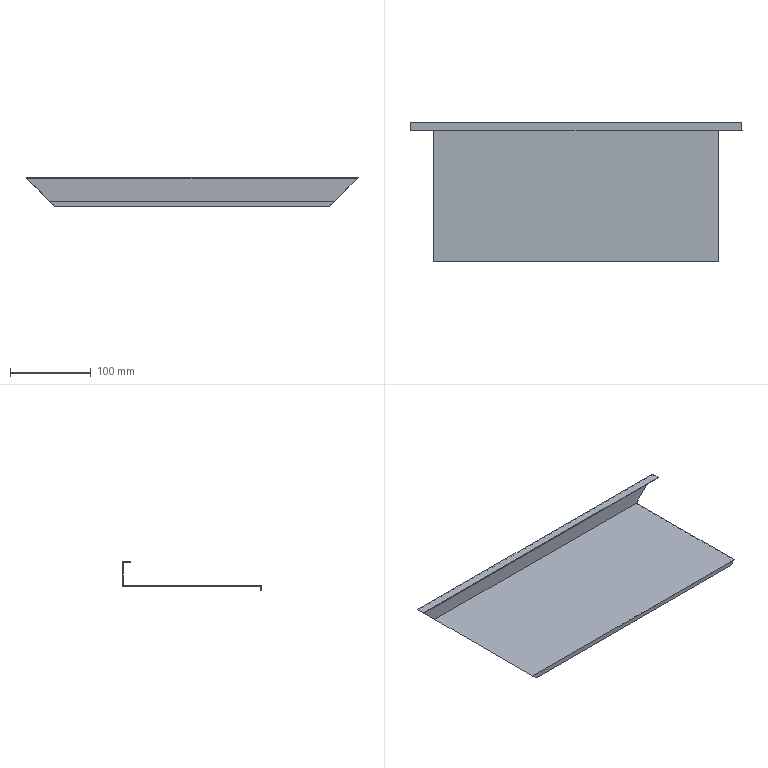Part | STEP file | 09-04 Inner side plate 1 | 1 solid | 12 faces | box 410 x 172 x 35 mm | volume 76827 mm3 | plane 12
STEP:
#1=CARTESIAN_POINT('',(0.,0.,0.));
#2=DIRECTION('',(0.,0.,1.));
#3=DIRECTION('',(1.,0.,0.));
#4=AXIS2_PLACEMENT_3D('',#1,#2,#3);
#5=CARTESIAN_POINT('',(381.,171.,1.));
#6=VERTEX_POINT('',#5);
#7=CARTESIAN_POINT('',(381.,0.,1.));
#8=VERTEX_POINT('',#7);
#9=CARTESIAN_POINT('',(381.,85.5,1.));
#10=DIRECTION('',(0.,-1.,0.));
#11=VECTOR('',#10,1.);
#12=LINE('',#9,#11);
#13=CARTESIAN_POINT('',(29.,0.,1.));
#14=DIRECTION('',(0.,0.,-1.));
#15=DIRECTION('',(0.,1.,0.));
#16=AXIS2_PLACEMENT_3D('',#13,#14,#15);
#17=PLANE('',#16);
#18=CARTESIAN_POINT('',(85.5,352.));
#19=DIRECTION('',(-1.,0.));
#20=VECTOR('',#19,1.);
#21=LINE('',#18,#20);
#22=(GEOMETRIC_REPRESENTATION_CONTEXT(2)PARAMETRIC_REPRESENTATION_CONTEXT()REPRESENTATION_CONTEXT('',''));
#23=DEFINITIONAL_REPRESENTATION('',(#21),#22);
#24=PCURVE('',#17,#23);
#25=CARTESIAN_POINT('',(375.,0.,-5.));
#26=DIRECTION('',(-0.7071,0.,0.7071));
#27=DIRECTION('',(0.7071,0.,0.7071));
#28=AXIS2_PLACEMENT_3D('',#25,#26,#27);
#29=PLANE('',#28);
#30=CARTESIAN_POINT('',(8.485,85.5));
#31=DIRECTION('',(0.,-1.));
#32=VECTOR('',#31,1.);
#33=LINE('',#30,#32);
#34=(GEOMETRIC_REPRESENTATION_CONTEXT(2)PARAMETRIC_REPRESENTATION_CONTEXT()REPRESENTATION_CONTEXT('',''));
#35=DEFINITIONAL_REPRESENTATION('',(#33),#34);
#36=PCURVE('',#29,#35);
#37=SURFACE_CURVE('',#12,(#24,#36),.PCURVE_S1.);
#38=EDGE_CURVE('',#6,#8,#37,.T.);
#39=ORIENTED_EDGE('',*,*,#38,.F.);
#40=CARTESIAN_POINT('',(29.,171.,1.));
#41=VERTEX_POINT('',#40);
#42=CARTESIAN_POINT('',(205.,171.,1.));
#43=DIRECTION('',(1.,0.,0.));
#44=VECTOR('',#43,1.);
#45=LINE('',#42,#44);
#46=CARTESIAN_POINT('',(171.,176.));
#47=DIRECTION('',(0.,1.));
#48=VECTOR('',#47,1.);
#49=LINE('',#46,#48);
#50=(GEOMETRIC_REPRESENTATION_CONTEXT(2)PARAMETRIC_REPRESENTATION_CONTEXT()REPRESENTATION_CONTEXT('',''));
#51=DEFINITIONAL_REPRESENTATION('',(#49),#50);
#52=PCURVE('',#17,#51);
#53=CARTESIAN_POINT('',(-1.448,171.,1.));
#54=DIRECTION('',(0.,1.,0.));
#55=DIRECTION('',(0.,0.,1.));
#56=AXIS2_PLACEMENT_3D('',#53,#54,#55);
#57=PLANE('',#56);
#58=CARTESIAN_POINT('',(0.,206.448));
#59=DIRECTION('',(0.,1.));
#60=VECTOR('',#59,1.);
#61=LINE('',#58,#60);
#62=(GEOMETRIC_REPRESENTATION_CONTEXT(2)PARAMETRIC_REPRESENTATION_CONTEXT()REPRESENTATION_CONTEXT('',''));
#63=DEFINITIONAL_REPRESENTATION('',(#61),#62);
#64=PCURVE('',#57,#63);
#65=SURFACE_CURVE('',#45,(#52,#64),.PCURVE_S1.);
#66=EDGE_CURVE('',#41,#6,#65,.T.);
#67=ORIENTED_EDGE('',*,*,#66,.F.);
#68=CARTESIAN_POINT('',(29.,0.,1.));
#69=VERTEX_POINT('',#68);
#70=CARTESIAN_POINT('',(29.,85.5,1.));
#71=DIRECTION('',(0.,1.,0.));
#72=VECTOR('',#71,1.);
#73=LINE('',#70,#72);
#74=CARTESIAN_POINT('',(85.5,0.));
#75=DIRECTION('',(1.,0.));
#76=VECTOR('',#75,1.);
#77=LINE('',#74,#76);
#78=(GEOMETRIC_REPRESENTATION_CONTEXT(2)PARAMETRIC_REPRESENTATION_CONTEXT()REPRESENTATION_CONTEXT('',''));
#79=DEFINITIONAL_REPRESENTATION('',(#77),#78);
#80=PCURVE('',#17,#79);
#81=CARTESIAN_POINT('',(0.,0.,30.));
#82=DIRECTION('',(0.7071,0.,0.7071));
#83=DIRECTION('',(0.7071,0.,-0.7071));
#84=AXIS2_PLACEMENT_3D('',#81,#82,#83);
#85=PLANE('',#84);
#86=CARTESIAN_POINT('',(41.012,85.5));
#87=DIRECTION('',(0.,1.));
#88=VECTOR('',#87,1.);
#89=LINE('',#86,#88);
#90=(GEOMETRIC_REPRESENTATION_CONTEXT(2)PARAMETRIC_REPRESENTATION_CONTEXT()REPRESENTATION_CONTEXT('',''));
#91=DEFINITIONAL_REPRESENTATION('',(#89),#90);
#92=PCURVE('',#85,#91);
#93=SURFACE_CURVE('',#73,(#80,#92),.PCURVE_S1.);
#94=EDGE_CURVE('',#69,#41,#93,.T.);
#95=ORIENTED_EDGE('',*,*,#94,.F.);
#96=CARTESIAN_POINT('',(205.,0.,1.));
#97=DIRECTION('',(-1.,0.,0.));
#98=VECTOR('',#97,1.);
#99=LINE('',#96,#98);
#100=CARTESIAN_POINT('',(0.,176.));
#101=DIRECTION('',(0.,-1.));
#102=VECTOR('',#101,1.);
#103=LINE('',#100,#102);
#104=(GEOMETRIC_REPRESENTATION_CONTEXT(2)PARAMETRIC_REPRESENTATION_CONTEXT()REPRESENTATION_CONTEXT('',''));
#105=DEFINITIONAL_REPRESENTATION('',(#103),#104);
#106=PCURVE('',#17,#105);
#107=CARTESIAN_POINT('',(26.888,0.,-5.));
#108=DIRECTION('',(0.,1.,0.));
#109=DIRECTION('',(0.,0.,1.));
#110=AXIS2_PLACEMENT_3D('',#107,#108,#109);
#111=PLANE('',#110);
#112=CARTESIAN_POINT('',(6.,178.112));
#113=DIRECTION('',(0.,-1.));
#114=VECTOR('',#113,1.);
#115=LINE('',#112,#114);
#116=(GEOMETRIC_REPRESENTATION_CONTEXT(2)PARAMETRIC_REPRESENTATION_CONTEXT()REPRESENTATION_CONTEXT('',''));
#117=DEFINITIONAL_REPRESENTATION('',(#115),#116);
#118=PCURVE('',#111,#117);
#119=SURFACE_CURVE('',#99,(#106,#118),.PCURVE_S1.);
#120=EDGE_CURVE('',#8,#69,#119,.T.);
#121=ORIENTED_EDGE('',*,*,#120,.F.);
#122=EDGE_LOOP('',(#39,#67,#95,#121));
#123=FACE_BOUND('',#122,.T.);
#124=ADVANCED_FACE('',(#123),#17,.F.);
#125=CARTESIAN_POINT('',(375.,0.,-5.));
#126=VERTEX_POINT('',#125);
#127=CARTESIAN_POINT('',(375.,0.,-5.));
#128=DIRECTION('',(-0.7071,0.,-0.7071));
#129=VECTOR('',#128,1.);
#130=LINE('',#127,#129);
#131=CARTESIAN_POINT('',(0.,348.112));
#132=DIRECTION('',(-0.7071,-0.7071));
#133=VECTOR('',#132,1.);
#134=LINE('',#131,#133);
#135=(GEOMETRIC_REPRESENTATION_CONTEXT(2)PARAMETRIC_REPRESENTATION_CONTEXT()REPRESENTATION_CONTEXT('',''));
#136=DEFINITIONAL_REPRESENTATION('',(#134),#135);
#137=PCURVE('',#111,#136);
#138=CARTESIAN_POINT('',(0.,0.));
#139=DIRECTION('',(-1.,0.));
#140=VECTOR('',#139,1.);
#141=LINE('',#138,#140);
#142=(GEOMETRIC_REPRESENTATION_CONTEXT(2)PARAMETRIC_REPRESENTATION_CONTEXT()REPRESENTATION_CONTEXT('',''));
#143=DEFINITIONAL_REPRESENTATION('',(#141),#142);
#144=PCURVE('',#29,#143);
#145=SURFACE_CURVE('',#130,(#137,#144),.PCURVE_S1.);
#146=EDGE_CURVE('',#8,#126,#145,.T.);
#147=ORIENTED_EDGE('',*,*,#146,.F.);
#148=ORIENTED_EDGE('',*,*,#120,.T.);
#149=CARTESIAN_POINT('',(35.,0.,-5.));
#150=VERTEX_POINT('',#149);
#151=CARTESIAN_POINT('',(0.,0.,30.));
#152=DIRECTION('',(-0.7071,0.,0.7071));
#153=VECTOR('',#152,1.);
#154=LINE('',#151,#153);
#155=CARTESIAN_POINT('',(35.,-26.888));
#156=DIRECTION('',(0.7071,-0.7071));
#157=VECTOR('',#156,1.);
#158=LINE('',#155,#157);
#159=(GEOMETRIC_REPRESENTATION_CONTEXT(2)PARAMETRIC_REPRESENTATION_CONTEXT()REPRESENTATION_CONTEXT('',''));
#160=DEFINITIONAL_REPRESENTATION('',(#158),#159);
#161=PCURVE('',#111,#160);
#162=CARTESIAN_POINT('',(0.,0.));
#163=DIRECTION('',(-1.,0.));
#164=VECTOR('',#163,1.);
#165=LINE('',#162,#164);
#166=(GEOMETRIC_REPRESENTATION_CONTEXT(2)PARAMETRIC_REPRESENTATION_CONTEXT()REPRESENTATION_CONTEXT('',''));
#167=DEFINITIONAL_REPRESENTATION('',(#165),#166);
#168=PCURVE('',#85,#167);
#169=SURFACE_CURVE('',#154,(#161,#168),.PCURVE_S1.);
#170=EDGE_CURVE('',#150,#69,#169,.T.);
#171=ORIENTED_EDGE('',*,*,#170,.F.);
#172=CARTESIAN_POINT('',(205.,0.,-5.));
#173=DIRECTION('',(-1.,0.,0.));
#174=VECTOR('',#173,1.);
#175=LINE('',#172,#174);
#176=CARTESIAN_POINT('',(0.,178.112));
#177=DIRECTION('',(0.,-1.));
#178=VECTOR('',#177,1.);
#179=LINE('',#176,#178);
#180=(GEOMETRIC_REPRESENTATION_CONTEXT(2)PARAMETRIC_REPRESENTATION_CONTEXT()REPRESENTATION_CONTEXT('',''));
#181=DEFINITIONAL_REPRESENTATION('',(#179),#180);
#182=PCURVE('',#111,#181);
#183=CARTESIAN_POINT('',(35.,0.,-5.));
#184=DIRECTION('',(0.,0.,1.));
#185=DIRECTION('',(1.,0.,0.));
#186=AXIS2_PLACEMENT_3D('',#183,#184,#185);
#187=PLANE('',#186);
#188=CARTESIAN_POINT('',(170.,0.));
#189=DIRECTION('',(-1.,0.));
#190=VECTOR('',#189,1.);
#191=LINE('',#188,#190);
#192=(GEOMETRIC_REPRESENTATION_CONTEXT(2)PARAMETRIC_REPRESENTATION_CONTEXT()REPRESENTATION_CONTEXT('',''));
#193=DEFINITIONAL_REPRESENTATION('',(#191),#192);
#194=PCURVE('',#187,#193);
#195=SURFACE_CURVE('',#175,(#182,#194),.PCURVE_S1.);
#196=EDGE_CURVE('',#126,#150,#195,.T.);
#197=ORIENTED_EDGE('',*,*,#196,.F.);
#198=EDGE_LOOP('',(#147,#148,#171,#197));
#199=FACE_BOUND('',#198,.T.);
#200=ADVANCED_FACE('',(#199),#111,.F.);
#201=CARTESIAN_POINT('',(410.,172.,30.));
#202=VERTEX_POINT('',#201);
#203=CARTESIAN_POINT('',(380.,172.,0.000000001));
#204=VERTEX_POINT('',#203);
#205=CARTESIAN_POINT('',(392.5,172.,12.5));
#206=DIRECTION('',(-0.7071,0.,-0.7071));
#207=VECTOR('',#206,1.);
#208=LINE('',#205,#207);
#209=CARTESIAN_POINT('',(24.749,172.));
#210=DIRECTION('',(-1.,0.));
#211=VECTOR('',#210,1.);
#212=LINE('',#209,#211);
#213=(GEOMETRIC_REPRESENTATION_CONTEXT(2)PARAMETRIC_REPRESENTATION_CONTEXT()REPRESENTATION_CONTEXT('',''));
#214=DEFINITIONAL_REPRESENTATION('',(#212),#213);
#215=PCURVE('',#29,#214);
#216=CARTESIAN_POINT('',(-2.46,172.,30.));
#217=DIRECTION('',(0.,-1.,0.));
#218=DIRECTION('',(0.,0.,-1.));
#219=AXIS2_PLACEMENT_3D('',#216,#217,#218);
#220=PLANE('',#219);
#221=CARTESIAN_POINT('',(17.5,394.96));
#222=DIRECTION('',(0.7071,-0.7071));
#223=VECTOR('',#222,1.);
#224=LINE('',#221,#223);
#225=(GEOMETRIC_REPRESENTATION_CONTEXT(2)PARAMETRIC_REPRESENTATION_CONTEXT()REPRESENTATION_CONTEXT('',''));
#226=DEFINITIONAL_REPRESENTATION('',(#224),#225);
#227=PCURVE('',#220,#226);
#228=SURFACE_CURVE('',#208,(#215,#227),.PCURVE_S1.);
#229=EDGE_CURVE('',#202,#204,#228,.T.);
#230=ORIENTED_EDGE('',*,*,#229,.F.);
#231=CARTESIAN_POINT('',(410.,162.,30.));
#232=VERTEX_POINT('',#231);
#233=CARTESIAN_POINT('',(410.,86.,30.));
#234=DIRECTION('',(0.,1.,0.));
#235=VECTOR('',#234,1.);
#236=LINE('',#233,#235);
#237=CARTESIAN_POINT('',(49.497,86.));
#238=DIRECTION('',(0.,1.));
#239=VECTOR('',#238,1.);
#240=LINE('',#237,#239);
#241=(GEOMETRIC_REPRESENTATION_CONTEXT(2)PARAMETRIC_REPRESENTATION_CONTEXT()REPRESENTATION_CONTEXT('',''));
#242=DEFINITIONAL_REPRESENTATION('',(#240),#241);
#243=PCURVE('',#29,#242);
#244=CARTESIAN_POINT('',(0.,162.,30.));
#245=DIRECTION('',(0.,0.,-1.));
#246=DIRECTION('',(0.,1.,0.));
#247=AXIS2_PLACEMENT_3D('',#244,#245,#246);
#248=PLANE('',#247);
#249=CARTESIAN_POINT('',(-76.,410.));
#250=DIRECTION('',(1.,0.));
#251=VECTOR('',#250,1.);
#252=LINE('',#249,#251);
#253=(GEOMETRIC_REPRESENTATION_CONTEXT(2)PARAMETRIC_REPRESENTATION_CONTEXT()REPRESENTATION_CONTEXT('',''));
#254=DEFINITIONAL_REPRESENTATION('',(#252),#253);
#255=PCURVE('',#248,#254);
#256=SURFACE_CURVE('',#236,(#243,#255),.PCURVE_S1.);
#257=EDGE_CURVE('',#232,#202,#256,.T.);
#258=ORIENTED_EDGE('',*,*,#257,.F.);
#259=CARTESIAN_POINT('',(409.,162.,29.));
#260=VERTEX_POINT('',#259);
#261=CARTESIAN_POINT('',(375.,162.,-5.));
#262=DIRECTION('',(-0.7071,0.,-0.7071));
#263=VECTOR('',#262,1.);
#264=LINE('',#261,#263);
#265=CARTESIAN_POINT('',(0.,162.));
#266=DIRECTION('',(-1.,0.));
#267=VECTOR('',#266,1.);
#268=LINE('',#265,#267);
#269=(GEOMETRIC_REPRESENTATION_CONTEXT(2)PARAMETRIC_REPRESENTATION_CONTEXT()REPRESENTATION_CONTEXT('',''));
#270=DEFINITIONAL_REPRESENTATION('',(#268),#269);
#271=PCURVE('',#29,#270);
#272=CARTESIAN_POINT('',(-2.46,162.,29.));
#273=DIRECTION('',(0.,1.,0.));
#274=DIRECTION('',(0.,0.,1.));
#275=AXIS2_PLACEMENT_3D('',#272,#273,#274);
#276=PLANE('',#275);
#277=CARTESIAN_POINT('',(-34.,377.46));
#278=DIRECTION('',(-0.7071,-0.7071));
#279=VECTOR('',#278,1.);
#280=LINE('',#277,#279);
#281=(GEOMETRIC_REPRESENTATION_CONTEXT(2)PARAMETRIC_REPRESENTATION_CONTEXT()REPRESENTATION_CONTEXT('',''));
#282=DEFINITIONAL_REPRESENTATION('',(#280),#281);
#283=PCURVE('',#276,#282);
#284=SURFACE_CURVE('',#264,(#271,#283),.PCURVE_S1.);
#285=EDGE_CURVE('',#232,#260,#284,.T.);
#286=ORIENTED_EDGE('',*,*,#285,.T.);
#287=CARTESIAN_POINT('',(409.,171.,29.));
#288=VERTEX_POINT('',#287);
#289=CARTESIAN_POINT('',(409.,86.,29.));
#290=DIRECTION('',(0.,-1.,0.));
#291=VECTOR('',#290,1.);
#292=LINE('',#289,#291);
#293=CARTESIAN_POINT('',(48.083,86.));
#294=DIRECTION('',(0.,-1.));
#295=VECTOR('',#294,1.);
#296=LINE('',#293,#295);
#297=(GEOMETRIC_REPRESENTATION_CONTEXT(2)PARAMETRIC_REPRESENTATION_CONTEXT()REPRESENTATION_CONTEXT('',''));
#298=DEFINITIONAL_REPRESENTATION('',(#296),#297);
#299=PCURVE('',#29,#298);
#300=CARTESIAN_POINT('',(1.,162.,29.));
#301=DIRECTION('',(0.,0.,1.));
#302=DIRECTION('',(1.,0.,0.));
#303=AXIS2_PLACEMENT_3D('',#300,#301,#302);
#304=PLANE('',#303);
#305=CARTESIAN_POINT('',(408.,-76.));
#306=DIRECTION('',(0.,-1.));
#307=VECTOR('',#306,1.);
#308=LINE('',#305,#307);
#309=(GEOMETRIC_REPRESENTATION_CONTEXT(2)PARAMETRIC_REPRESENTATION_CONTEXT()REPRESENTATION_CONTEXT('',''));
#310=DEFINITIONAL_REPRESENTATION('',(#308),#309);
#311=PCURVE('',#304,#310);
#312=SURFACE_CURVE('',#292,(#299,#311),.PCURVE_S1.);
#313=EDGE_CURVE('',#288,#260,#312,.T.);
#314=ORIENTED_EDGE('',*,*,#313,.F.);
#315=CARTESIAN_POINT('',(392.5,171.,12.5));
#316=DIRECTION('',(0.7071,0.,0.7071));
#317=VECTOR('',#316,1.);
#318=LINE('',#315,#317);
#319=CARTESIAN_POINT('',(24.749,171.));
#320=DIRECTION('',(1.,0.));
#321=VECTOR('',#320,1.);
#322=LINE('',#319,#321);
#323=(GEOMETRIC_REPRESENTATION_CONTEXT(2)PARAMETRIC_REPRESENTATION_CONTEXT()REPRESENTATION_CONTEXT('',''));
#324=DEFINITIONAL_REPRESENTATION('',(#322),#323);
#325=PCURVE('',#29,#324);
#326=CARTESIAN_POINT('',(11.5,393.948));
#327=DIRECTION('',(0.7071,0.7071));
#328=VECTOR('',#327,1.);
#329=LINE('',#326,#328);
#330=(GEOMETRIC_REPRESENTATION_CONTEXT(2)PARAMETRIC_REPRESENTATION_CONTEXT()REPRESENTATION_CONTEXT('',''));
#331=DEFINITIONAL_REPRESENTATION('',(#329),#330);
#332=PCURVE('',#57,#331);
#333=SURFACE_CURVE('',#318,(#325,#332),.PCURVE_S1.);
#334=EDGE_CURVE('',#6,#288,#333,.T.);
#335=ORIENTED_EDGE('',*,*,#334,.F.);
#336=ORIENTED_EDGE('',*,*,#38,.T.);
#337=ORIENTED_EDGE('',*,*,#146,.T.);
#338=CARTESIAN_POINT('',(375.,1.,-5.));
#339=VERTEX_POINT('',#338);
#340=CARTESIAN_POINT('',(375.,86.,-5.));
#341=DIRECTION('',(0.,-1.,0.));
#342=VECTOR('',#341,1.);
#343=LINE('',#340,#342);
#344=CARTESIAN_POINT('',(0.,86.));
#345=DIRECTION('',(0.,-1.));
#346=VECTOR('',#345,1.);
#347=LINE('',#344,#346);
#348=(GEOMETRIC_REPRESENTATION_CONTEXT(2)PARAMETRIC_REPRESENTATION_CONTEXT()REPRESENTATION_CONTEXT('',''));
#349=DEFINITIONAL_REPRESENTATION('',(#347),#348);
#350=PCURVE('',#29,#349);
#351=CARTESIAN_POINT('',(340.,86.));
#352=DIRECTION('',(0.,-1.));
#353=VECTOR('',#352,1.);
#354=LINE('',#351,#353);
#355=(GEOMETRIC_REPRESENTATION_CONTEXT(2)PARAMETRIC_REPRESENTATION_CONTEXT()REPRESENTATION_CONTEXT('',''));
#356=DEFINITIONAL_REPRESENTATION('',(#354),#355);
#357=PCURVE('',#187,#356);
#358=SURFACE_CURVE('',#343,(#350,#357),.PCURVE_S1.);
#359=EDGE_CURVE('',#339,#126,#358,.T.);
#360=ORIENTED_EDGE('',*,*,#359,.F.);
#361=CARTESIAN_POINT('',(380.,1.,0.000000001));
#362=VERTEX_POINT('',#361);
#363=CARTESIAN_POINT('',(392.5,1.,12.5));
#364=DIRECTION('',(-0.7071,0.,-0.7071));
#365=VECTOR('',#364,1.);
#366=LINE('',#363,#365);
#367=CARTESIAN_POINT('',(24.749,1.));
#368=DIRECTION('',(-1.,0.));
#369=VECTOR('',#368,1.);
#370=LINE('',#367,#369);
#371=(GEOMETRIC_REPRESENTATION_CONTEXT(2)PARAMETRIC_REPRESENTATION_CONTEXT()REPRESENTATION_CONTEXT('',''));
#372=DEFINITIONAL_REPRESENTATION('',(#370),#371);
#373=PCURVE('',#29,#372);
#374=CARTESIAN_POINT('',(27.9,1.,0.));
#375=DIRECTION('',(0.,-1.,0.));
#376=DIRECTION('',(0.,0.,-1.));
#377=AXIS2_PLACEMENT_3D('',#374,#375,#376);
#378=PLANE('',#377);
#379=CARTESIAN_POINT('',(-12.5,364.6));
#380=DIRECTION('',(0.7071,-0.7071));
#381=VECTOR('',#380,1.);
#382=LINE('',#379,#381);
#383=(GEOMETRIC_REPRESENTATION_CONTEXT(2)PARAMETRIC_REPRESENTATION_CONTEXT()REPRESENTATION_CONTEXT('',''));
#384=DEFINITIONAL_REPRESENTATION('',(#382),#383);
#385=PCURVE('',#378,#384);
#386=SURFACE_CURVE('',#366,(#373,#385),.PCURVE_S1.);
#387=EDGE_CURVE('',#362,#339,#386,.T.);
#388=ORIENTED_EDGE('',*,*,#387,.F.);
#389=CARTESIAN_POINT('',(380.,86.,0.000000005));
#390=DIRECTION('',(0.,-1.,0.));
#391=VECTOR('',#390,1.);
#392=LINE('',#389,#391);
#393=CARTESIAN_POINT('',(7.071,86.));
#394=DIRECTION('',(0.,-1.));
#395=VECTOR('',#394,1.);
#396=LINE('',#393,#395);
#397=(GEOMETRIC_REPRESENTATION_CONTEXT(2)PARAMETRIC_REPRESENTATION_CONTEXT()REPRESENTATION_CONTEXT('',''));
#398=DEFINITIONAL_REPRESENTATION('',(#396),#397);
#399=PCURVE('',#29,#398);
#400=CARTESIAN_POINT('',(30.,172.,0.));
#401=DIRECTION('',(0.,0.,1.));
#402=DIRECTION('',(0.,-1.,0.));
#403=AXIS2_PLACEMENT_3D('',#400,#401,#402);
#404=PLANE('',#403);
#405=CARTESIAN_POINT('',(86.,350.));
#406=DIRECTION('',(1.,0.));
#407=VECTOR('',#406,1.);
#408=LINE('',#405,#407);
#409=(GEOMETRIC_REPRESENTATION_CONTEXT(2)PARAMETRIC_REPRESENTATION_CONTEXT()REPRESENTATION_CONTEXT('',''));
#410=DEFINITIONAL_REPRESENTATION('',(#408),#409);
#411=PCURVE('',#404,#410);
#412=SURFACE_CURVE('',#392,(#399,#411),.PCURVE_S1.);
#413=EDGE_CURVE('',#204,#362,#412,.T.);
#414=ORIENTED_EDGE('',*,*,#413,.F.);
#415=EDGE_LOOP('',(#230,#258,#286,#314,#335,#336,#337,#360,#388,#414));
#416=FACE_BOUND('',#415,.T.);
#417=ADVANCED_FACE('',(#416),#29,.F.);
#418=ORIENTED_EDGE('',*,*,#334,.T.);
#419=CARTESIAN_POINT('',(1.,171.,29.));
#420=VERTEX_POINT('',#419);
#421=CARTESIAN_POINT('',(205.,171.,29.));
#422=DIRECTION('',(1.,0.,0.));
#423=VECTOR('',#422,1.);
#424=LINE('',#421,#423);
#425=CARTESIAN_POINT('',(28.,206.448));
#426=DIRECTION('',(0.,1.));
#427=VECTOR('',#426,1.);
#428=LINE('',#425,#427);
#429=(GEOMETRIC_REPRESENTATION_CONTEXT(2)PARAMETRIC_REPRESENTATION_CONTEXT()REPRESENTATION_CONTEXT('',''));
#430=DEFINITIONAL_REPRESENTATION('',(#428),#429);
#431=PCURVE('',#57,#430);
#432=CARTESIAN_POINT('',(204.,9.));
#433=DIRECTION('',(1.,0.));
#434=VECTOR('',#433,1.);
#435=LINE('',#432,#434);
#436=(GEOMETRIC_REPRESENTATION_CONTEXT(2)PARAMETRIC_REPRESENTATION_CONTEXT()REPRESENTATION_CONTEXT('',''));
#437=DEFINITIONAL_REPRESENTATION('',(#435),#436);
#438=PCURVE('',#304,#437);
#439=SURFACE_CURVE('',#424,(#431,#438),.PCURVE_S1.);
#440=EDGE_CURVE('',#420,#288,#439,.T.);
#441=ORIENTED_EDGE('',*,*,#440,.F.);
#442=CARTESIAN_POINT('',(0.,171.,30.));
#443=DIRECTION('',(-0.7071,0.,0.7071));
#444=VECTOR('',#443,1.);
#445=LINE('',#442,#444);
#446=CARTESIAN_POINT('',(29.,1.448));
#447=DIRECTION('',(0.7071,-0.7071));
#448=VECTOR('',#447,1.);
#449=LINE('',#446,#448);
#450=(GEOMETRIC_REPRESENTATION_CONTEXT(2)PARAMETRIC_REPRESENTATION_CONTEXT()REPRESENTATION_CONTEXT('',''));
#451=DEFINITIONAL_REPRESENTATION('',(#449),#450);
#452=PCURVE('',#57,#451);
#453=CARTESIAN_POINT('',(0.,171.));
#454=DIRECTION('',(-1.,0.));
#455=VECTOR('',#454,1.);
#456=LINE('',#453,#455);
#457=(GEOMETRIC_REPRESENTATION_CONTEXT(2)PARAMETRIC_REPRESENTATION_CONTEXT()REPRESENTATION_CONTEXT('',''));
#458=DEFINITIONAL_REPRESENTATION('',(#456),#457);
#459=PCURVE('',#85,#458);
#460=SURFACE_CURVE('',#445,(#452,#459),.PCURVE_S1.);
#461=EDGE_CURVE('',#41,#420,#460,.T.);
#462=ORIENTED_EDGE('',*,*,#461,.F.);
#463=ORIENTED_EDGE('',*,*,#66,.T.);
#464=EDGE_LOOP('',(#418,#441,#462,#463));
#465=FACE_BOUND('',#464,.T.);
#466=ADVANCED_FACE('',(#465),#57,.F.);
#467=ORIENTED_EDGE('',*,*,#170,.T.);
#468=ORIENTED_EDGE('',*,*,#94,.T.);
#469=ORIENTED_EDGE('',*,*,#461,.T.);
#470=CARTESIAN_POINT('',(1.,162.,29.));
#471=VERTEX_POINT('',#470);
#472=CARTESIAN_POINT('',(1.,86.,29.));
#473=DIRECTION('',(0.,1.,0.));
#474=VECTOR('',#473,1.);
#475=LINE('',#472,#474);
#476=CARTESIAN_POINT('',(1.414,86.));
#477=DIRECTION('',(0.,1.));
#478=VECTOR('',#477,1.);
#479=LINE('',#476,#478);
#480=(GEOMETRIC_REPRESENTATION_CONTEXT(2)PARAMETRIC_REPRESENTATION_CONTEXT()REPRESENTATION_CONTEXT('',''));
#481=DEFINITIONAL_REPRESENTATION('',(#479),#480);
#482=PCURVE('',#85,#481);
#483=CARTESIAN_POINT('',(0.000000015,-76.));
#484=DIRECTION('',(0.,1.));
#485=VECTOR('',#484,1.);
#486=LINE('',#483,#485);
#487=(GEOMETRIC_REPRESENTATION_CONTEXT(2)PARAMETRIC_REPRESENTATION_CONTEXT()REPRESENTATION_CONTEXT('',''));
#488=DEFINITIONAL_REPRESENTATION('',(#486),#487);
#489=PCURVE('',#304,#488);
#490=SURFACE_CURVE('',#475,(#482,#489),.PCURVE_S1.);
#491=EDGE_CURVE('',#471,#420,#490,.T.);
#492=ORIENTED_EDGE('',*,*,#491,.F.);
#493=CARTESIAN_POINT('',(0.,162.,30.));
#494=VERTEX_POINT('',#493);
#495=CARTESIAN_POINT('',(0.,162.,30.));
#496=DIRECTION('',(-0.7071,0.,0.7071));
#497=VECTOR('',#496,1.);
#498=LINE('',#495,#497);
#499=CARTESIAN_POINT('',(0.,162.));
#500=DIRECTION('',(-1.,0.));
#501=VECTOR('',#500,1.);
#502=LINE('',#499,#501);
#503=(GEOMETRIC_REPRESENTATION_CONTEXT(2)PARAMETRIC_REPRESENTATION_CONTEXT()REPRESENTATION_CONTEXT('',''));
#504=DEFINITIONAL_REPRESENTATION('',(#502),#503);
#505=PCURVE('',#85,#504);
#506=CARTESIAN_POINT('',(1.,2.46));
#507=DIRECTION('',(0.7071,-0.7071));
#508=VECTOR('',#507,1.);
#509=LINE('',#506,#508);
#510=(GEOMETRIC_REPRESENTATION_CONTEXT(2)PARAMETRIC_REPRESENTATION_CONTEXT()REPRESENTATION_CONTEXT('',''));
#511=DEFINITIONAL_REPRESENTATION('',(#509),#510);
#512=PCURVE('',#276,#511);
#513=SURFACE_CURVE('',#498,(#505,#512),.PCURVE_S1.);
#514=EDGE_CURVE('',#471,#494,#513,.T.);
#515=ORIENTED_EDGE('',*,*,#514,.T.);
#516=CARTESIAN_POINT('',(0.000000051,172.,30.));
#517=VERTEX_POINT('',#516);
#518=CARTESIAN_POINT('',(0.,86.,30.));
#519=DIRECTION('',(0.,-1.,0.));
#520=VECTOR('',#519,1.);
#521=LINE('',#518,#520);
#522=CARTESIAN_POINT('',(0.,86.));
#523=DIRECTION('',(0.,-1.));
#524=VECTOR('',#523,1.);
#525=LINE('',#522,#524);
#526=(GEOMETRIC_REPRESENTATION_CONTEXT(2)PARAMETRIC_REPRESENTATION_CONTEXT()REPRESENTATION_CONTEXT('',''));
#527=DEFINITIONAL_REPRESENTATION('',(#525),#526);
#528=PCURVE('',#85,#527);
#529=CARTESIAN_POINT('',(-76.,0.));
#530=DIRECTION('',(-1.,0.));
#531=VECTOR('',#530,1.);
#532=LINE('',#529,#531);
#533=(GEOMETRIC_REPRESENTATION_CONTEXT(2)PARAMETRIC_REPRESENTATION_CONTEXT()REPRESENTATION_CONTEXT('',''));
#534=DEFINITIONAL_REPRESENTATION('',(#532),#533);
#535=PCURVE('',#248,#534);
#536=SURFACE_CURVE('',#521,(#528,#535),.PCURVE_S1.);
#537=EDGE_CURVE('',#517,#494,#536,.T.);
#538=ORIENTED_EDGE('',*,*,#537,.F.);
#539=CARTESIAN_POINT('',(30.,172.,0.000000001));
#540=VERTEX_POINT('',#539);
#541=CARTESIAN_POINT('',(17.5,172.,12.5));
#542=DIRECTION('',(-0.7071,0.,0.7071));
#543=VECTOR('',#542,1.);
#544=LINE('',#541,#543);
#545=CARTESIAN_POINT('',(24.749,172.));
#546=DIRECTION('',(-1.,0.));
#547=VECTOR('',#546,1.);
#548=LINE('',#545,#547);
#549=(GEOMETRIC_REPRESENTATION_CONTEXT(2)PARAMETRIC_REPRESENTATION_CONTEXT()REPRESENTATION_CONTEXT('',''));
#550=DEFINITIONAL_REPRESENTATION('',(#548),#549);
#551=PCURVE('',#85,#550);
#552=CARTESIAN_POINT('',(17.5,19.96));
#553=DIRECTION('',(-0.7071,-0.7071));
#554=VECTOR('',#553,1.);
#555=LINE('',#552,#554);
#556=(GEOMETRIC_REPRESENTATION_CONTEXT(2)PARAMETRIC_REPRESENTATION_CONTEXT()REPRESENTATION_CONTEXT('',''));
#557=DEFINITIONAL_REPRESENTATION('',(#555),#556);
#558=PCURVE('',#220,#557);
#559=SURFACE_CURVE('',#544,(#551,#558),.PCURVE_S1.);
#560=EDGE_CURVE('',#540,#517,#559,.T.);
#561=ORIENTED_EDGE('',*,*,#560,.F.);
#562=CARTESIAN_POINT('',(30.,1.,0.000000001));
#563=VERTEX_POINT('',#562);
#564=CARTESIAN_POINT('',(30.,86.,0.000000005));
#565=DIRECTION('',(0.,1.,0.));
#566=VECTOR('',#565,1.);
#567=LINE('',#564,#566);
#568=CARTESIAN_POINT('',(42.426,86.));
#569=DIRECTION('',(0.,1.));
#570=VECTOR('',#569,1.);
#571=LINE('',#568,#570);
#572=(GEOMETRIC_REPRESENTATION_CONTEXT(2)PARAMETRIC_REPRESENTATION_CONTEXT()REPRESENTATION_CONTEXT('',''));
#573=DEFINITIONAL_REPRESENTATION('',(#571),#572);
#574=PCURVE('',#85,#573);
#575=CARTESIAN_POINT('',(86.,-0.000000005));
#576=DIRECTION('',(-1.,0.));
#577=VECTOR('',#576,1.);
#578=LINE('',#575,#577);
#579=(GEOMETRIC_REPRESENTATION_CONTEXT(2)PARAMETRIC_REPRESENTATION_CONTEXT()REPRESENTATION_CONTEXT('',''));
#580=DEFINITIONAL_REPRESENTATION('',(#578),#579);
#581=PCURVE('',#404,#580);
#582=SURFACE_CURVE('',#567,(#574,#581),.PCURVE_S1.);
#583=EDGE_CURVE('',#563,#540,#582,.T.);
#584=ORIENTED_EDGE('',*,*,#583,.F.);
#585=CARTESIAN_POINT('',(35.,1.,-5.));
#586=VERTEX_POINT('',#585);
#587=CARTESIAN_POINT('',(17.5,1.,12.5));
#588=DIRECTION('',(-0.7071,0.,0.7071));
#589=VECTOR('',#588,1.);
#590=LINE('',#587,#589);
#591=CARTESIAN_POINT('',(24.749,1.));
#592=DIRECTION('',(-1.,0.));
#593=VECTOR('',#592,1.);
#594=LINE('',#591,#593);
#595=(GEOMETRIC_REPRESENTATION_CONTEXT(2)PARAMETRIC_REPRESENTATION_CONTEXT()REPRESENTATION_CONTEXT('',''));
#596=DEFINITIONAL_REPRESENTATION('',(#594),#595);
#597=PCURVE('',#85,#596);
#598=CARTESIAN_POINT('',(-12.5,-10.4));
#599=DIRECTION('',(-0.7071,-0.7071));
#600=VECTOR('',#599,1.);
#601=LINE('',#598,#600);
#602=(GEOMETRIC_REPRESENTATION_CONTEXT(2)PARAMETRIC_REPRESENTATION_CONTEXT()REPRESENTATION_CONTEXT('',''));
#603=DEFINITIONAL_REPRESENTATION('',(#601),#602);
#604=PCURVE('',#378,#603);
#605=SURFACE_CURVE('',#590,(#597,#604),.PCURVE_S1.);
#606=EDGE_CURVE('',#586,#563,#605,.T.);
#607=ORIENTED_EDGE('',*,*,#606,.F.);
#608=CARTESIAN_POINT('',(35.,86.,-5.));
#609=DIRECTION('',(0.,1.,0.));
#610=VECTOR('',#609,1.);
#611=LINE('',#608,#610);
#612=CARTESIAN_POINT('',(49.497,86.));
#613=DIRECTION('',(0.,1.));
#614=VECTOR('',#613,1.);
#615=LINE('',#612,#614);
#616=(GEOMETRIC_REPRESENTATION_CONTEXT(2)PARAMETRIC_REPRESENTATION_CONTEXT()REPRESENTATION_CONTEXT('',''));
#617=DEFINITIONAL_REPRESENTATION('',(#615),#616);
#618=PCURVE('',#85,#617);
#619=CARTESIAN_POINT('',(0.,86.));
#620=DIRECTION('',(0.,1.));
#621=VECTOR('',#620,1.);
#622=LINE('',#619,#621);
#623=(GEOMETRIC_REPRESENTATION_CONTEXT(2)PARAMETRIC_REPRESENTATION_CONTEXT()REPRESENTATION_CONTEXT('',''));
#624=DEFINITIONAL_REPRESENTATION('',(#622),#623);
#625=PCURVE('',#187,#624);
#626=SURFACE_CURVE('',#611,(#618,#625),.PCURVE_S1.);
#627=EDGE_CURVE('',#150,#586,#626,.T.);
#628=ORIENTED_EDGE('',*,*,#627,.F.);
#629=EDGE_LOOP('',(#467,#468,#469,#492,#515,#538,#561,#584,#607,#628));
#630=FACE_BOUND('',#629,.T.);
#631=ADVANCED_FACE('',(#630),#85,.F.);
#632=ORIENTED_EDGE('',*,*,#359,.T.);
#633=ORIENTED_EDGE('',*,*,#196,.T.);
#634=ORIENTED_EDGE('',*,*,#627,.T.);
#635=CARTESIAN_POINT('',(205.,1.,-5.));
#636=DIRECTION('',(-1.,0.,0.));
#637=VECTOR('',#636,1.);
#638=LINE('',#635,#637);
#639=CARTESIAN_POINT('',(170.,1.));
#640=DIRECTION('',(-1.,0.));
#641=VECTOR('',#640,1.);
#642=LINE('',#639,#641);
#643=(GEOMETRIC_REPRESENTATION_CONTEXT(2)PARAMETRIC_REPRESENTATION_CONTEXT()REPRESENTATION_CONTEXT('',''));
#644=DEFINITIONAL_REPRESENTATION('',(#642),#643);
#645=PCURVE('',#187,#644);
#646=CARTESIAN_POINT('',(5.,177.1));
#647=DIRECTION('',(0.,-1.));
#648=VECTOR('',#647,1.);
#649=LINE('',#646,#648);
#650=(GEOMETRIC_REPRESENTATION_CONTEXT(2)PARAMETRIC_REPRESENTATION_CONTEXT()REPRESENTATION_CONTEXT('',''));
#651=DEFINITIONAL_REPRESENTATION('',(#649),#650);
#652=PCURVE('',#378,#651);
#653=SURFACE_CURVE('',#638,(#645,#652),.PCURVE_S1.);
#654=EDGE_CURVE('',#339,#586,#653,.T.);
#655=ORIENTED_EDGE('',*,*,#654,.F.);
#656=EDGE_LOOP('',(#632,#633,#634,#655));
#657=FACE_BOUND('',#656,.T.);
#658=ADVANCED_FACE('',(#657),#187,.F.);
#659=ORIENTED_EDGE('',*,*,#413,.T.);
#660=CARTESIAN_POINT('',(205.,1.,0.));
#661=DIRECTION('',(1.,0.,0.));
#662=VECTOR('',#661,1.);
#663=LINE('',#660,#662);
#664=CARTESIAN_POINT('',(171.,175.));
#665=DIRECTION('',(0.,1.));
#666=VECTOR('',#665,1.);
#667=LINE('',#664,#666);
#668=(GEOMETRIC_REPRESENTATION_CONTEXT(2)PARAMETRIC_REPRESENTATION_CONTEXT()REPRESENTATION_CONTEXT('',''));
#669=DEFINITIONAL_REPRESENTATION('',(#667),#668);
#670=PCURVE('',#404,#669);
#671=CARTESIAN_POINT('',(0.,177.1));
#672=DIRECTION('',(0.,1.));
#673=VECTOR('',#672,1.);
#674=LINE('',#671,#673);
#675=(GEOMETRIC_REPRESENTATION_CONTEXT(2)PARAMETRIC_REPRESENTATION_CONTEXT()REPRESENTATION_CONTEXT('',''));
#676=DEFINITIONAL_REPRESENTATION('',(#674),#675);
#677=PCURVE('',#378,#676);
#678=SURFACE_CURVE('',#663,(#670,#677),.PCURVE_S1.);
#679=EDGE_CURVE('',#563,#362,#678,.T.);
#680=ORIENTED_EDGE('',*,*,#679,.F.);
#681=ORIENTED_EDGE('',*,*,#583,.T.);
#682=CARTESIAN_POINT('',(205.,172.,0.));
#683=DIRECTION('',(-1.,0.,0.));
#684=VECTOR('',#683,1.);
#685=LINE('',#682,#684);
#686=CARTESIAN_POINT('',(0.,175.));
#687=DIRECTION('',(0.,-1.));
#688=VECTOR('',#687,1.);
#689=LINE('',#686,#688);
#690=(GEOMETRIC_REPRESENTATION_CONTEXT(2)PARAMETRIC_REPRESENTATION_CONTEXT()REPRESENTATION_CONTEXT('',''));
#691=DEFINITIONAL_REPRESENTATION('',(#689),#690);
#692=PCURVE('',#404,#691);
#693=CARTESIAN_POINT('',(30.,207.46));
#694=DIRECTION('',(0.,-1.));
#695=VECTOR('',#694,1.);
#696=LINE('',#693,#695);
#697=(GEOMETRIC_REPRESENTATION_CONTEXT(2)PARAMETRIC_REPRESENTATION_CONTEXT()REPRESENTATION_CONTEXT('',''));
#698=DEFINITIONAL_REPRESENTATION('',(#696),#697);
#699=PCURVE('',#220,#698);
#700=SURFACE_CURVE('',#685,(#692,#699),.PCURVE_S1.);
#701=EDGE_CURVE('',#204,#540,#700,.T.);
#702=ORIENTED_EDGE('',*,*,#701,.F.);
#703=EDGE_LOOP('',(#659,#680,#681,#702));
#704=FACE_BOUND('',#703,.T.);
#705=ADVANCED_FACE('',(#704),#404,.F.);
#706=ORIENTED_EDGE('',*,*,#229,.T.);
#707=ORIENTED_EDGE('',*,*,#701,.T.);
#708=ORIENTED_EDGE('',*,*,#560,.T.);
#709=CARTESIAN_POINT('',(205.,172.,30.));
#710=DIRECTION('',(-1.,0.,0.));
#711=VECTOR('',#710,1.);
#712=LINE('',#709,#711);
#713=CARTESIAN_POINT('',(0.,207.46));
#714=DIRECTION('',(0.,-1.));
#715=VECTOR('',#714,1.);
#716=LINE('',#713,#715);
#717=(GEOMETRIC_REPRESENTATION_CONTEXT(2)PARAMETRIC_REPRESENTATION_CONTEXT()REPRESENTATION_CONTEXT('',''));
#718=DEFINITIONAL_REPRESENTATION('',(#716),#717);
#719=PCURVE('',#220,#718);
#720=CARTESIAN_POINT('',(10.,205.));
#721=DIRECTION('',(0.,-1.));
#722=VECTOR('',#721,1.);
#723=LINE('',#720,#722);
#724=(GEOMETRIC_REPRESENTATION_CONTEXT(2)PARAMETRIC_REPRESENTATION_CONTEXT()REPRESENTATION_CONTEXT('',''));
#725=DEFINITIONAL_REPRESENTATION('',(#723),#724);
#726=PCURVE('',#248,#725);
#727=SURFACE_CURVE('',#712,(#719,#726),.PCURVE_S1.);
#728=EDGE_CURVE('',#202,#517,#727,.T.);
#729=ORIENTED_EDGE('',*,*,#728,.F.);
#730=EDGE_LOOP('',(#706,#707,#708,#729));
#731=FACE_BOUND('',#730,.T.);
#732=ADVANCED_FACE('',(#731),#220,.F.);
#733=CARTESIAN_POINT('',(205.,162.,30.));
#734=DIRECTION('',(-1.,0.,0.));
#735=VECTOR('',#734,1.);
#736=LINE('',#733,#735);
#737=CARTESIAN_POINT('',(0.,205.));
#738=DIRECTION('',(0.,-1.));
#739=VECTOR('',#738,1.);
#740=LINE('',#737,#739);
#741=(GEOMETRIC_REPRESENTATION_CONTEXT(2)PARAMETRIC_REPRESENTATION_CONTEXT()REPRESENTATION_CONTEXT('',''));
#742=DEFINITIONAL_REPRESENTATION('',(#740),#741);
#743=PCURVE('',#248,#742);
#744=CARTESIAN_POINT('',(1.,207.46));
#745=DIRECTION('',(0.,-1.));
#746=VECTOR('',#745,1.);
#747=LINE('',#744,#746);
#748=(GEOMETRIC_REPRESENTATION_CONTEXT(2)PARAMETRIC_REPRESENTATION_CONTEXT()REPRESENTATION_CONTEXT('',''));
#749=DEFINITIONAL_REPRESENTATION('',(#747),#748);
#750=PCURVE('',#276,#749);
#751=SURFACE_CURVE('',#736,(#743,#750),.PCURVE_S1.);
#752=EDGE_CURVE('',#232,#494,#751,.T.);
#753=ORIENTED_EDGE('',*,*,#752,.F.);
#754=ORIENTED_EDGE('',*,*,#257,.T.);
#755=ORIENTED_EDGE('',*,*,#728,.T.);
#756=ORIENTED_EDGE('',*,*,#537,.T.);
#757=EDGE_LOOP('',(#753,#754,#755,#756));
#758=FACE_BOUND('',#757,.T.);
#759=ADVANCED_FACE('',(#758),#248,.F.);
#760=ORIENTED_EDGE('',*,*,#313,.T.);
#761=CARTESIAN_POINT('',(205.,162.,29.));
#762=DIRECTION('',(1.,0.,0.));
#763=VECTOR('',#762,1.);
#764=LINE('',#761,#763);
#765=CARTESIAN_POINT('',(204.,0.));
#766=DIRECTION('',(1.,0.));
#767=VECTOR('',#766,1.);
#768=LINE('',#765,#767);
#769=(GEOMETRIC_REPRESENTATION_CONTEXT(2)PARAMETRIC_REPRESENTATION_CONTEXT()REPRESENTATION_CONTEXT('',''));
#770=DEFINITIONAL_REPRESENTATION('',(#768),#769);
#771=PCURVE('',#304,#770);
#772=CARTESIAN_POINT('',(0.,207.46));
#773=DIRECTION('',(0.,1.));
#774=VECTOR('',#773,1.);
#775=LINE('',#772,#774);
#776=(GEOMETRIC_REPRESENTATION_CONTEXT(2)PARAMETRIC_REPRESENTATION_CONTEXT()REPRESENTATION_CONTEXT('',''));
#777=DEFINITIONAL_REPRESENTATION('',(#775),#776);
#778=PCURVE('',#276,#777);
#779=SURFACE_CURVE('',#764,(#771,#778),.PCURVE_S1.);
#780=EDGE_CURVE('',#471,#260,#779,.T.);
#781=ORIENTED_EDGE('',*,*,#780,.F.);
#782=ORIENTED_EDGE('',*,*,#491,.T.);
#783=ORIENTED_EDGE('',*,*,#440,.T.);
#784=EDGE_LOOP('',(#760,#781,#782,#783));
#785=FACE_BOUND('',#784,.T.);
#786=ADVANCED_FACE('',(#785),#304,.F.);
#787=ORIENTED_EDGE('',*,*,#387,.T.);
#788=ORIENTED_EDGE('',*,*,#654,.T.);
#789=ORIENTED_EDGE('',*,*,#606,.T.);
#790=ORIENTED_EDGE('',*,*,#679,.T.);
#791=EDGE_LOOP('',(#787,#788,#789,#790));
#792=FACE_BOUND('',#791,.T.);
#793=ADVANCED_FACE('',(#792),#378,.F.);
#794=ORIENTED_EDGE('',*,*,#285,.F.);
#795=ORIENTED_EDGE('',*,*,#752,.T.);
#796=ORIENTED_EDGE('',*,*,#514,.F.);
#797=ORIENTED_EDGE('',*,*,#780,.T.);
#798=EDGE_LOOP('',(#794,#795,#796,#797));
#799=FACE_BOUND('',#798,.T.);
#800=ADVANCED_FACE('',(#799),#276,.F.);
#801=CLOSED_SHELL('',(#124,#200,#417,#466,#631,#658,#705,#732,#759,#786,#793,#800));
#802=MANIFOLD_SOLID_BREP('',#801);
#803=(LENGTH_UNIT()NAMED_UNIT(*)SI_UNIT(.MILLI.,.METRE.));
#804=UNCERTAINTY_MEASURE_WITH_UNIT(LENGTH_MEASURE(0.0000001),#803,'','');
#805=(NAMED_UNIT(*)PLANE_ANGLE_UNIT()SI_UNIT($,.RADIAN.));
#806=(NAMED_UNIT(*)SI_UNIT($,.STERADIAN.)SOLID_ANGLE_UNIT());
#807=(GEOMETRIC_REPRESENTATION_CONTEXT(3)GLOBAL_UNCERTAINTY_ASSIGNED_CONTEXT((#804))GLOBAL_UNIT_ASSIGNED_CONTEXT((#803,#805,#806))REPRESENTATION_CONTEXT('',''));
#808=ADVANCED_BREP_SHAPE_REPRESENTATION('',(#4,#802),#807);